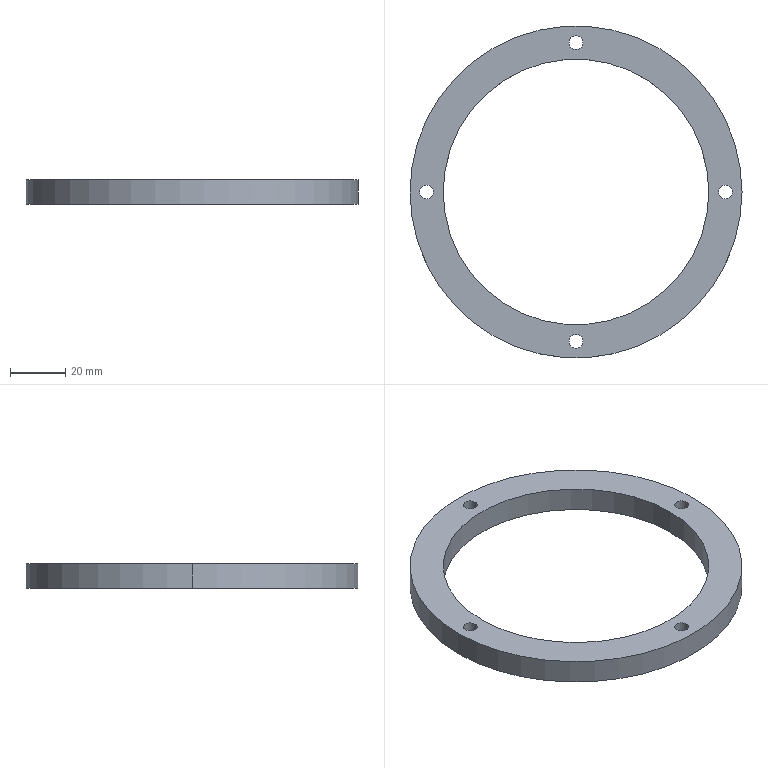Part | SolidWorks | features BaseBody 1 | 1 solid | 14 faces | box 120 x 120 x 9 mm | volume 35937 mm3 | cylinder 12 | plane 2 | commonest cylinder face diameters 5 x8 96 x2 120 x2
STEP:
#1=CARTESIAN_POINT('',(-51.5,0.,9.));
#2=VERTEX_POINT('',#1);
#3=CARTESIAN_POINT('',(-56.5,0.,9.));
#4=VERTEX_POINT('',#3);
#5=CARTESIAN_POINT('',(-54.,0.,9.));
#6=DIRECTION('',(0.,0.,-1.));
#7=DIRECTION('',(-1.,0.,0.));
#8=AXIS2_PLACEMENT_3D('',#5,#6,#7);
#9=CIRCLE('',#8,2.5);
#10=EDGE_CURVE('',#2,#4,#9,.T.);
#11=ORIENTED_EDGE('',*,*,#10,.F.);
#12=CARTESIAN_POINT('',(-51.5,0.,0.));
#13=VERTEX_POINT('',#12);
#14=CARTESIAN_POINT('',(-51.5,0.,9.));
#15=DIRECTION('',(0.,0.,-1.));
#16=VECTOR('',#15,1000.);
#17=LINE('',#14,#16);
#18=EDGE_CURVE('',#2,#13,#17,.T.);
#19=ORIENTED_EDGE('',*,*,#18,.T.);
#20=CARTESIAN_POINT('',(-56.5,0.,0.));
#21=VERTEX_POINT('',#20);
#22=CARTESIAN_POINT('',(-54.,0.,0.));
#23=DIRECTION('',(0.,0.,1.));
#24=DIRECTION('',(-1.,0.,0.));
#25=AXIS2_PLACEMENT_3D('',#22,#23,#24);
#26=CIRCLE('',#25,2.5);
#27=EDGE_CURVE('',#21,#13,#26,.T.);
#28=ORIENTED_EDGE('',*,*,#27,.F.);
#29=CARTESIAN_POINT('',(-56.5,0.,9.));
#30=DIRECTION('',(0.,0.,-1.));
#31=VECTOR('',#30,1000.);
#32=LINE('',#29,#31);
#33=EDGE_CURVE('',#4,#21,#32,.T.);
#34=ORIENTED_EDGE('',*,*,#33,.F.);
#35=EDGE_LOOP('',(#11,#19,#28,#34));
#36=FACE_OUTER_BOUND('',#35,.T.);
#37=CARTESIAN_POINT('',(-54.,0.,9.));
#38=DIRECTION('',(0.,0.,-1.));
#39=DIRECTION('',(-1.,0.,0.));
#40=AXIS2_PLACEMENT_3D('',#37,#38,#39);
#41=CYLINDRICAL_SURFACE('',#40,2.5);
#42=ADVANCED_FACE('',(#36),#41,.F.);
#43=CARTESIAN_POINT('',(56.5,0.,9.));
#44=VERTEX_POINT('',#43);
#45=CARTESIAN_POINT('',(51.5,0.,9.));
#46=VERTEX_POINT('',#45);
#47=CARTESIAN_POINT('',(54.,0.,9.));
#48=DIRECTION('',(0.,0.,-1.));
#49=DIRECTION('',(-1.,0.,0.));
#50=AXIS2_PLACEMENT_3D('',#47,#48,#49);
#51=CIRCLE('',#50,2.5);
#52=EDGE_CURVE('',#44,#46,#51,.T.);
#53=ORIENTED_EDGE('',*,*,#52,.F.);
#54=CARTESIAN_POINT('',(56.5,0.,0.));
#55=VERTEX_POINT('',#54);
#56=CARTESIAN_POINT('',(56.5,0.,9.));
#57=DIRECTION('',(0.,0.,-1.));
#58=VECTOR('',#57,1000.);
#59=LINE('',#56,#58);
#60=EDGE_CURVE('',#44,#55,#59,.T.);
#61=ORIENTED_EDGE('',*,*,#60,.T.);
#62=CARTESIAN_POINT('',(51.5,0.,0.));
#63=VERTEX_POINT('',#62);
#64=CARTESIAN_POINT('',(54.,0.,0.));
#65=DIRECTION('',(0.,0.,1.));
#66=DIRECTION('',(-1.,0.,0.));
#67=AXIS2_PLACEMENT_3D('',#64,#65,#66);
#68=CIRCLE('',#67,2.5);
#69=EDGE_CURVE('',#63,#55,#68,.T.);
#70=ORIENTED_EDGE('',*,*,#69,.F.);
#71=CARTESIAN_POINT('',(51.5,0.,9.));
#72=DIRECTION('',(0.,0.,-1.));
#73=VECTOR('',#72,1000.);
#74=LINE('',#71,#73);
#75=EDGE_CURVE('',#46,#63,#74,.T.);
#76=ORIENTED_EDGE('',*,*,#75,.F.);
#77=EDGE_LOOP('',(#53,#61,#70,#76));
#78=FACE_OUTER_BOUND('',#77,.T.);
#79=CARTESIAN_POINT('',(54.,0.,9.));
#80=DIRECTION('',(0.,0.,-1.));
#81=DIRECTION('',(-1.,0.,0.));
#82=AXIS2_PLACEMENT_3D('',#79,#80,#81);
#83=CYLINDRICAL_SURFACE('',#82,2.5);
#84=ADVANCED_FACE('',(#78),#83,.F.);
#85=CARTESIAN_POINT('',(48.,0.,9.));
#86=VERTEX_POINT('',#85);
#87=CARTESIAN_POINT('',(-48.,0.,9.));
#88=VERTEX_POINT('',#87);
#89=CARTESIAN_POINT('',(0.,0.,9.));
#90=DIRECTION('',(0.,0.,-1.));
#91=DIRECTION('',(-1.,0.,0.));
#92=AXIS2_PLACEMENT_3D('',#89,#90,#91);
#93=CIRCLE('',#92,48.);
#94=EDGE_CURVE('',#86,#88,#93,.T.);
#95=ORIENTED_EDGE('',*,*,#94,.F.);
#96=CARTESIAN_POINT('',(48.,0.,0.));
#97=VERTEX_POINT('',#96);
#98=CARTESIAN_POINT('',(48.,0.,9.));
#99=DIRECTION('',(0.,0.,-1.));
#100=VECTOR('',#99,1000.);
#101=LINE('',#98,#100);
#102=EDGE_CURVE('',#86,#97,#101,.T.);
#103=ORIENTED_EDGE('',*,*,#102,.T.);
#104=CARTESIAN_POINT('',(-48.,0.,0.));
#105=VERTEX_POINT('',#104);
#106=CARTESIAN_POINT('',(0.,0.,0.));
#107=DIRECTION('',(0.,0.,1.));
#108=DIRECTION('',(-1.,0.,0.));
#109=AXIS2_PLACEMENT_3D('',#106,#107,#108);
#110=CIRCLE('',#109,48.);
#111=EDGE_CURVE('',#105,#97,#110,.T.);
#112=ORIENTED_EDGE('',*,*,#111,.F.);
#113=CARTESIAN_POINT('',(-48.,0.,9.));
#114=DIRECTION('',(0.,0.,-1.));
#115=VECTOR('',#114,1000.);
#116=LINE('',#113,#115);
#117=EDGE_CURVE('',#88,#105,#116,.T.);
#118=ORIENTED_EDGE('',*,*,#117,.F.);
#119=EDGE_LOOP('',(#95,#103,#112,#118));
#120=FACE_OUTER_BOUND('',#119,.T.);
#121=CARTESIAN_POINT('',(0.,0.,9.));
#122=DIRECTION('',(0.,0.,-1.));
#123=DIRECTION('',(-1.,0.,0.));
#124=AXIS2_PLACEMENT_3D('',#121,#122,#123);
#125=CYLINDRICAL_SURFACE('',#124,48.);
#126=ADVANCED_FACE('',(#120),#125,.F.);
#127=CARTESIAN_POINT('',(60.,0.,9.));
#128=VERTEX_POINT('',#127);
#129=CARTESIAN_POINT('',(-60.,0.,9.));
#130=VERTEX_POINT('',#129);
#131=CARTESIAN_POINT('',(0.,0.,9.));
#132=DIRECTION('',(0.,0.,1.));
#133=DIRECTION('',(-1.,0.,0.));
#134=AXIS2_PLACEMENT_3D('',#131,#132,#133);
#135=CIRCLE('',#134,60.);
#136=EDGE_CURVE('',#128,#130,#135,.T.);
#137=ORIENTED_EDGE('',*,*,#136,.F.);
#138=CARTESIAN_POINT('',(60.,0.,0.));
#139=VERTEX_POINT('',#138);
#140=CARTESIAN_POINT('',(60.,0.,9.));
#141=DIRECTION('',(0.,0.,-1.));
#142=VECTOR('',#141,1000.);
#143=LINE('',#140,#142);
#144=EDGE_CURVE('',#128,#139,#143,.T.);
#145=ORIENTED_EDGE('',*,*,#144,.T.);
#146=CARTESIAN_POINT('',(-60.,0.,0.));
#147=VERTEX_POINT('',#146);
#148=CARTESIAN_POINT('',(0.,0.,0.));
#149=DIRECTION('',(0.,0.,1.));
#150=DIRECTION('',(-1.,0.,0.));
#151=AXIS2_PLACEMENT_3D('',#148,#149,#150);
#152=CIRCLE('',#151,60.);
#153=EDGE_CURVE('',#139,#147,#152,.T.);
#154=ORIENTED_EDGE('',*,*,#153,.T.);
#155=CARTESIAN_POINT('',(-60.,0.,9.));
#156=DIRECTION('',(0.,0.,-1.));
#157=VECTOR('',#156,1000.);
#158=LINE('',#155,#157);
#159=EDGE_CURVE('',#130,#147,#158,.T.);
#160=ORIENTED_EDGE('',*,*,#159,.F.);
#161=EDGE_LOOP('',(#137,#145,#154,#160));
#162=FACE_OUTER_BOUND('',#161,.T.);
#163=CARTESIAN_POINT('',(0.,0.,9.));
#164=DIRECTION('',(0.,0.,-1.));
#165=DIRECTION('',(-1.,0.,0.));
#166=AXIS2_PLACEMENT_3D('',#163,#164,#165);
#167=CYLINDRICAL_SURFACE('',#166,60.);
#168=ADVANCED_FACE('',(#162),#167,.T.);
#169=CARTESIAN_POINT('',(2.5,54.,9.));
#170=VERTEX_POINT('',#169);
#171=CARTESIAN_POINT('',(-2.5,54.,9.));
#172=VERTEX_POINT('',#171);
#173=CARTESIAN_POINT('',(0.,54.,9.));
#174=DIRECTION('',(0.,0.,-1.));
#175=DIRECTION('',(-1.,0.,0.));
#176=AXIS2_PLACEMENT_3D('',#173,#174,#175);
#177=CIRCLE('',#176,2.5);
#178=EDGE_CURVE('',#170,#172,#177,.T.);
#179=ORIENTED_EDGE('',*,*,#178,.F.);
#180=CARTESIAN_POINT('',(2.5,54.,0.));
#181=VERTEX_POINT('',#180);
#182=CARTESIAN_POINT('',(2.5,54.,9.));
#183=DIRECTION('',(0.,0.,-1.));
#184=VECTOR('',#183,1000.);
#185=LINE('',#182,#184);
#186=EDGE_CURVE('',#170,#181,#185,.T.);
#187=ORIENTED_EDGE('',*,*,#186,.T.);
#188=CARTESIAN_POINT('',(-2.5,54.,0.));
#189=VERTEX_POINT('',#188);
#190=CARTESIAN_POINT('',(0.,54.,0.));
#191=DIRECTION('',(0.,0.,1.));
#192=DIRECTION('',(-1.,0.,0.));
#193=AXIS2_PLACEMENT_3D('',#190,#191,#192);
#194=CIRCLE('',#193,2.5);
#195=EDGE_CURVE('',#189,#181,#194,.T.);
#196=ORIENTED_EDGE('',*,*,#195,.F.);
#197=CARTESIAN_POINT('',(-2.5,54.,9.));
#198=DIRECTION('',(0.,0.,-1.));
#199=VECTOR('',#198,1000.);
#200=LINE('',#197,#199);
#201=EDGE_CURVE('',#172,#189,#200,.T.);
#202=ORIENTED_EDGE('',*,*,#201,.F.);
#203=EDGE_LOOP('',(#179,#187,#196,#202));
#204=FACE_OUTER_BOUND('',#203,.T.);
#205=CARTESIAN_POINT('',(0.,54.,9.));
#206=DIRECTION('',(0.,0.,-1.));
#207=DIRECTION('',(-1.,0.,0.));
#208=AXIS2_PLACEMENT_3D('',#205,#206,#207);
#209=CYLINDRICAL_SURFACE('',#208,2.5);
#210=ADVANCED_FACE('',(#204),#209,.F.);
#211=CARTESIAN_POINT('',(2.5,-54.,9.));
#212=VERTEX_POINT('',#211);
#213=CARTESIAN_POINT('',(-2.5,-54.,9.));
#214=VERTEX_POINT('',#213);
#215=CARTESIAN_POINT('',(0.,-54.,9.));
#216=DIRECTION('',(0.,0.,-1.));
#217=DIRECTION('',(-1.,0.,0.));
#218=AXIS2_PLACEMENT_3D('',#215,#216,#217);
#219=CIRCLE('',#218,2.5);
#220=EDGE_CURVE('',#212,#214,#219,.T.);
#221=ORIENTED_EDGE('',*,*,#220,.F.);
#222=CARTESIAN_POINT('',(2.5,-54.,0.));
#223=VERTEX_POINT('',#222);
#224=CARTESIAN_POINT('',(2.5,-54.,9.));
#225=DIRECTION('',(0.,0.,-1.));
#226=VECTOR('',#225,1000.);
#227=LINE('',#224,#226);
#228=EDGE_CURVE('',#212,#223,#227,.T.);
#229=ORIENTED_EDGE('',*,*,#228,.T.);
#230=CARTESIAN_POINT('',(-2.5,-54.,0.));
#231=VERTEX_POINT('',#230);
#232=CARTESIAN_POINT('',(0.,-54.,0.));
#233=DIRECTION('',(0.,0.,1.));
#234=DIRECTION('',(-1.,0.,0.));
#235=AXIS2_PLACEMENT_3D('',#232,#233,#234);
#236=CIRCLE('',#235,2.5);
#237=EDGE_CURVE('',#231,#223,#236,.T.);
#238=ORIENTED_EDGE('',*,*,#237,.F.);
#239=CARTESIAN_POINT('',(-2.5,-54.,9.));
#240=DIRECTION('',(0.,0.,-1.));
#241=VECTOR('',#240,1000.);
#242=LINE('',#239,#241);
#243=EDGE_CURVE('',#214,#231,#242,.T.);
#244=ORIENTED_EDGE('',*,*,#243,.F.);
#245=EDGE_LOOP('',(#221,#229,#238,#244));
#246=FACE_OUTER_BOUND('',#245,.T.);
#247=CARTESIAN_POINT('',(0.,-54.,9.));
#248=DIRECTION('',(0.,0.,-1.));
#249=DIRECTION('',(-1.,0.,0.));
#250=AXIS2_PLACEMENT_3D('',#247,#248,#249);
#251=CYLINDRICAL_SURFACE('',#250,2.5);
#252=ADVANCED_FACE('',(#246),#251,.F.);
#253=CARTESIAN_POINT('',(-54.,0.,9.));
#254=DIRECTION('',(0.,0.,-1.));
#255=DIRECTION('',(-1.,0.,0.));
#256=AXIS2_PLACEMENT_3D('',#253,#254,#255);
#257=CIRCLE('',#256,2.5);
#258=EDGE_CURVE('',#4,#2,#257,.T.);
#259=ORIENTED_EDGE('',*,*,#258,.T.);
#260=ORIENTED_EDGE('',*,*,#10,.T.);
#261=EDGE_LOOP('',(#259,#260));
#262=FACE_BOUND('',#261,.T.);
#263=CARTESIAN_POINT('',(54.,0.,9.));
#264=DIRECTION('',(0.,0.,-1.));
#265=DIRECTION('',(-1.,0.,0.));
#266=AXIS2_PLACEMENT_3D('',#263,#264,#265);
#267=CIRCLE('',#266,2.5);
#268=EDGE_CURVE('',#46,#44,#267,.T.);
#269=ORIENTED_EDGE('',*,*,#268,.T.);
#270=ORIENTED_EDGE('',*,*,#52,.T.);
#271=EDGE_LOOP('',(#269,#270));
#272=FACE_BOUND('',#271,.T.);
#273=CARTESIAN_POINT('',(0.,0.,9.));
#274=DIRECTION('',(0.,0.,-1.));
#275=DIRECTION('',(-1.,0.,0.));
#276=AXIS2_PLACEMENT_3D('',#273,#274,#275);
#277=CIRCLE('',#276,48.);
#278=EDGE_CURVE('',#88,#86,#277,.T.);
#279=ORIENTED_EDGE('',*,*,#278,.T.);
#280=ORIENTED_EDGE('',*,*,#94,.T.);
#281=EDGE_LOOP('',(#279,#280));
#282=FACE_BOUND('',#281,.T.);
#283=CARTESIAN_POINT('',(0.,0.,9.));
#284=DIRECTION('',(0.,0.,1.));
#285=DIRECTION('',(-1.,0.,0.));
#286=AXIS2_PLACEMENT_3D('',#283,#284,#285);
#287=CIRCLE('',#286,60.);
#288=EDGE_CURVE('',#130,#128,#287,.T.);
#289=ORIENTED_EDGE('',*,*,#288,.T.);
#290=ORIENTED_EDGE('',*,*,#136,.T.);
#291=EDGE_LOOP('',(#289,#290));
#292=FACE_OUTER_BOUND('',#291,.T.);
#293=CARTESIAN_POINT('',(0.,54.,9.));
#294=DIRECTION('',(0.,0.,-1.));
#295=DIRECTION('',(-1.,0.,0.));
#296=AXIS2_PLACEMENT_3D('',#293,#294,#295);
#297=CIRCLE('',#296,2.5);
#298=EDGE_CURVE('',#172,#170,#297,.T.);
#299=ORIENTED_EDGE('',*,*,#298,.T.);
#300=ORIENTED_EDGE('',*,*,#178,.T.);
#301=EDGE_LOOP('',(#299,#300));
#302=FACE_BOUND('',#301,.T.);
#303=CARTESIAN_POINT('',(0.,-54.,9.));
#304=DIRECTION('',(0.,0.,-1.));
#305=DIRECTION('',(-1.,0.,0.));
#306=AXIS2_PLACEMENT_3D('',#303,#304,#305);
#307=CIRCLE('',#306,2.5);
#308=EDGE_CURVE('',#214,#212,#307,.T.);
#309=ORIENTED_EDGE('',*,*,#308,.T.);
#310=ORIENTED_EDGE('',*,*,#220,.T.);
#311=EDGE_LOOP('',(#309,#310));
#312=FACE_BOUND('',#311,.T.);
#313=CARTESIAN_POINT('',(0.,0.,9.));
#314=DIRECTION('',(0.,0.,1.));
#315=DIRECTION('',(1.,0.,0.));
#316=AXIS2_PLACEMENT_3D('',#313,#314,#315);
#317=PLANE('',#316);
#318=ADVANCED_FACE('',(#262,#272,#282,#292,#302,#312),#317,.T.);
#319=ORIENTED_EDGE('',*,*,#18,.F.);
#320=ORIENTED_EDGE('',*,*,#258,.F.);
#321=ORIENTED_EDGE('',*,*,#33,.T.);
#322=CARTESIAN_POINT('',(-54.,0.,0.));
#323=DIRECTION('',(0.,0.,1.));
#324=DIRECTION('',(-1.,0.,0.));
#325=AXIS2_PLACEMENT_3D('',#322,#323,#324);
#326=CIRCLE('',#325,2.5);
#327=EDGE_CURVE('',#13,#21,#326,.T.);
#328=ORIENTED_EDGE('',*,*,#327,.F.);
#329=EDGE_LOOP('',(#319,#320,#321,#328));
#330=FACE_OUTER_BOUND('',#329,.T.);
#331=CARTESIAN_POINT('',(-54.,0.,9.));
#332=DIRECTION('',(0.,0.,-1.));
#333=DIRECTION('',(-1.,0.,0.));
#334=AXIS2_PLACEMENT_3D('',#331,#332,#333);
#335=CYLINDRICAL_SURFACE('',#334,2.5);
#336=ADVANCED_FACE('',(#330),#335,.F.);
#337=ORIENTED_EDGE('',*,*,#60,.F.);
#338=ORIENTED_EDGE('',*,*,#268,.F.);
#339=ORIENTED_EDGE('',*,*,#75,.T.);
#340=CARTESIAN_POINT('',(54.,0.,0.));
#341=DIRECTION('',(0.,0.,1.));
#342=DIRECTION('',(-1.,0.,0.));
#343=AXIS2_PLACEMENT_3D('',#340,#341,#342);
#344=CIRCLE('',#343,2.5);
#345=EDGE_CURVE('',#55,#63,#344,.T.);
#346=ORIENTED_EDGE('',*,*,#345,.F.);
#347=EDGE_LOOP('',(#337,#338,#339,#346));
#348=FACE_OUTER_BOUND('',#347,.T.);
#349=CARTESIAN_POINT('',(54.,0.,9.));
#350=DIRECTION('',(0.,0.,-1.));
#351=DIRECTION('',(-1.,0.,0.));
#352=AXIS2_PLACEMENT_3D('',#349,#350,#351);
#353=CYLINDRICAL_SURFACE('',#352,2.5);
#354=ADVANCED_FACE('',(#348),#353,.F.);
#355=ORIENTED_EDGE('',*,*,#102,.F.);
#356=ORIENTED_EDGE('',*,*,#278,.F.);
#357=ORIENTED_EDGE('',*,*,#117,.T.);
#358=CARTESIAN_POINT('',(0.,0.,0.));
#359=DIRECTION('',(0.,0.,1.));
#360=DIRECTION('',(-1.,0.,0.));
#361=AXIS2_PLACEMENT_3D('',#358,#359,#360);
#362=CIRCLE('',#361,48.);
#363=EDGE_CURVE('',#97,#105,#362,.T.);
#364=ORIENTED_EDGE('',*,*,#363,.F.);
#365=EDGE_LOOP('',(#355,#356,#357,#364));
#366=FACE_OUTER_BOUND('',#365,.T.);
#367=CARTESIAN_POINT('',(0.,0.,9.));
#368=DIRECTION('',(0.,0.,-1.));
#369=DIRECTION('',(-1.,0.,0.));
#370=AXIS2_PLACEMENT_3D('',#367,#368,#369);
#371=CYLINDRICAL_SURFACE('',#370,48.);
#372=ADVANCED_FACE('',(#366),#371,.F.);
#373=ORIENTED_EDGE('',*,*,#144,.F.);
#374=ORIENTED_EDGE('',*,*,#288,.F.);
#375=ORIENTED_EDGE('',*,*,#159,.T.);
#376=CARTESIAN_POINT('',(0.,0.,0.));
#377=DIRECTION('',(0.,0.,1.));
#378=DIRECTION('',(-1.,0.,0.));
#379=AXIS2_PLACEMENT_3D('',#376,#377,#378);
#380=CIRCLE('',#379,60.);
#381=EDGE_CURVE('',#147,#139,#380,.T.);
#382=ORIENTED_EDGE('',*,*,#381,.T.);
#383=EDGE_LOOP('',(#373,#374,#375,#382));
#384=FACE_OUTER_BOUND('',#383,.T.);
#385=CARTESIAN_POINT('',(0.,0.,9.));
#386=DIRECTION('',(0.,0.,-1.));
#387=DIRECTION('',(-1.,0.,0.));
#388=AXIS2_PLACEMENT_3D('',#385,#386,#387);
#389=CYLINDRICAL_SURFACE('',#388,60.);
#390=ADVANCED_FACE('',(#384),#389,.T.);
#391=ORIENTED_EDGE('',*,*,#186,.F.);
#392=ORIENTED_EDGE('',*,*,#298,.F.);
#393=ORIENTED_EDGE('',*,*,#201,.T.);
#394=CARTESIAN_POINT('',(0.,54.,0.));
#395=DIRECTION('',(0.,0.,1.));
#396=DIRECTION('',(-1.,0.,0.));
#397=AXIS2_PLACEMENT_3D('',#394,#395,#396);
#398=CIRCLE('',#397,2.5);
#399=EDGE_CURVE('',#181,#189,#398,.T.);
#400=ORIENTED_EDGE('',*,*,#399,.F.);
#401=EDGE_LOOP('',(#391,#392,#393,#400));
#402=FACE_OUTER_BOUND('',#401,.T.);
#403=CARTESIAN_POINT('',(0.,54.,9.));
#404=DIRECTION('',(0.,0.,-1.));
#405=DIRECTION('',(-1.,0.,0.));
#406=AXIS2_PLACEMENT_3D('',#403,#404,#405);
#407=CYLINDRICAL_SURFACE('',#406,2.5);
#408=ADVANCED_FACE('',(#402),#407,.F.);
#409=ORIENTED_EDGE('',*,*,#228,.F.);
#410=ORIENTED_EDGE('',*,*,#308,.F.);
#411=ORIENTED_EDGE('',*,*,#243,.T.);
#412=CARTESIAN_POINT('',(0.,-54.,0.));
#413=DIRECTION('',(0.,0.,1.));
#414=DIRECTION('',(-1.,0.,0.));
#415=AXIS2_PLACEMENT_3D('',#412,#413,#414);
#416=CIRCLE('',#415,2.5);
#417=EDGE_CURVE('',#223,#231,#416,.T.);
#418=ORIENTED_EDGE('',*,*,#417,.F.);
#419=EDGE_LOOP('',(#409,#410,#411,#418));
#420=FACE_OUTER_BOUND('',#419,.T.);
#421=CARTESIAN_POINT('',(0.,-54.,9.));
#422=DIRECTION('',(0.,0.,-1.));
#423=DIRECTION('',(-1.,0.,0.));
#424=AXIS2_PLACEMENT_3D('',#421,#422,#423);
#425=CYLINDRICAL_SURFACE('',#424,2.5);
#426=ADVANCED_FACE('',(#420),#425,.F.);
#427=ORIENTED_EDGE('',*,*,#27,.T.);
#428=ORIENTED_EDGE('',*,*,#327,.T.);
#429=EDGE_LOOP('',(#427,#428));
#430=FACE_BOUND('',#429,.T.);
#431=ORIENTED_EDGE('',*,*,#237,.T.);
#432=ORIENTED_EDGE('',*,*,#417,.T.);
#433=EDGE_LOOP('',(#431,#432));
#434=FACE_BOUND('',#433,.T.);
#435=ORIENTED_EDGE('',*,*,#69,.T.);
#436=ORIENTED_EDGE('',*,*,#345,.T.);
#437=EDGE_LOOP('',(#435,#436));
#438=FACE_BOUND('',#437,.T.);
#439=ORIENTED_EDGE('',*,*,#195,.T.);
#440=ORIENTED_EDGE('',*,*,#399,.T.);
#441=EDGE_LOOP('',(#439,#440));
#442=FACE_BOUND('',#441,.T.);
#443=ORIENTED_EDGE('',*,*,#111,.T.);
#444=ORIENTED_EDGE('',*,*,#363,.T.);
#445=EDGE_LOOP('',(#443,#444));
#446=FACE_BOUND('',#445,.T.);
#447=ORIENTED_EDGE('',*,*,#381,.F.);
#448=ORIENTED_EDGE('',*,*,#153,.F.);
#449=EDGE_LOOP('',(#447,#448));
#450=FACE_OUTER_BOUND('',#449,.T.);
#451=CARTESIAN_POINT('',(0.,0.,0.));
#452=DIRECTION('',(0.,0.,1.));
#453=DIRECTION('',(1.,0.,0.));
#454=AXIS2_PLACEMENT_3D('',#451,#452,#453);
#455=PLANE('',#454);
#456=ADVANCED_FACE('',(#430,#434,#438,#442,#446,#450),#455,.F.);
#457=CLOSED_SHELL('',(#42,#84,#126,#168,#210,#252,#318,#336,#354,#372,#390,#408,#426,#456));
#458=MANIFOLD_SOLID_BREP('',#457);
#459=CARTESIAN_POINT('',(0.,0.,0.));
#460=DIRECTION('',(0.,0.,1.));
#461=DIRECTION('',(1.,0.,0.));
#462=AXIS2_PLACEMENT_3D('',#459,#460,#461);
#463=(LENGTH_UNIT()NAMED_UNIT(*)SI_UNIT(.MILLI.,.METRE.));
#464=UNCERTAINTY_MEASURE_WITH_UNIT(LENGTH_MEASURE(0.00001),#463,'','');
#465=(NAMED_UNIT(*)PLANE_ANGLE_UNIT()SI_UNIT($,.RADIAN.));
#466=(NAMED_UNIT(*)SI_UNIT($,.STERADIAN.)SOLID_ANGLE_UNIT());
#467=(GEOMETRIC_REPRESENTATION_CONTEXT(3)GLOBAL_UNCERTAINTY_ASSIGNED_CONTEXT((#464))GLOBAL_UNIT_ASSIGNED_CONTEXT((#463,#465,#466))REPRESENTATION_CONTEXT('',''));
#468=ADVANCED_BREP_SHAPE_REPRESENTATION('',(#458,#462),#467);